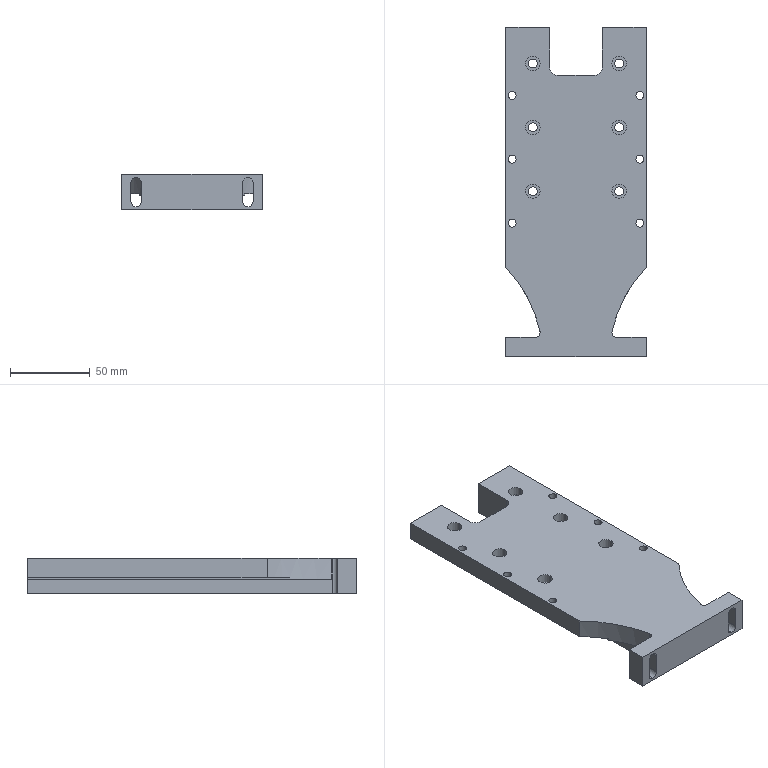Part | STEP file | Printing fixing plate | 1 solid | 85 faces | box 88 x 206 x 22 mm | volume 274808 mm3 | cylinder 51 | plane 32 | cone 2 | commonest cylinder face diameters 5 x12 5.5 x12 9 x12 6.5 x6 6 x3 6.8 x2